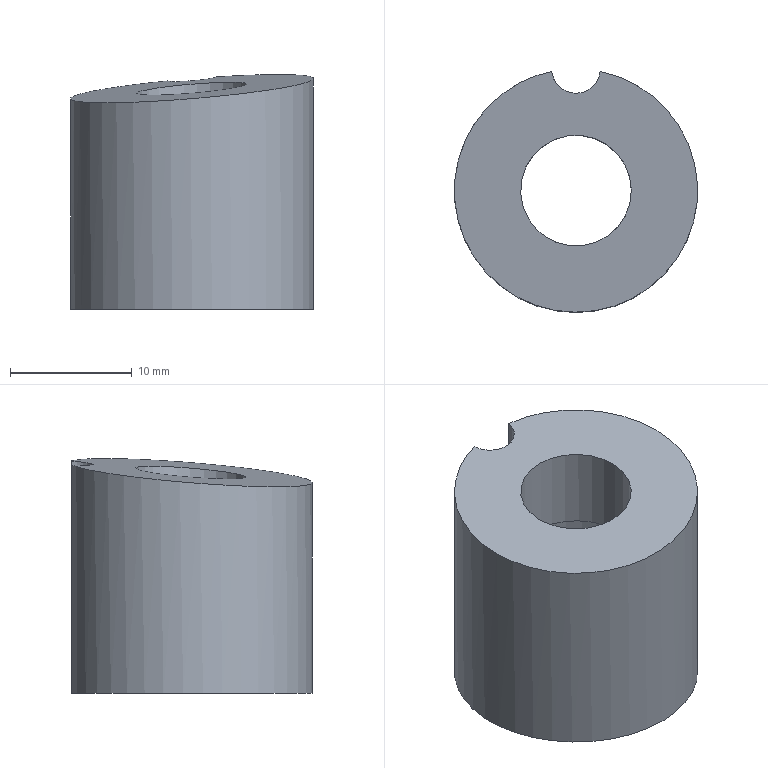Part | NX | features EKSD 20-20-10.10 2 | 1 solid | 7 faces | box 20 x 19.8 x 19.32 mm | volume 3694 mm3 | cylinder 4 | plane 3 | commonest cylinder face diameters 4 x1 9.1 x1 12.6 x1 20 x1
STEP:
#1=CARTESIAN_POINT('',(773.57,7.852,-2.));
#2=VERTEX_POINT('',#1);
#3=CARTESIAN_POINT('',(777.55,7.852,-2.));
#4=VERTEX_POINT('',#3);
#5=CARTESIAN_POINT('',(775.56,8.052,-2.));
#6=DIRECTION('',(0.,0.,1.));
#7=DIRECTION('',(1.,0.,0.));
#8=AXIS2_PLACEMENT_3D('',#5,#6,#7);
#9=CIRCLE('',#8,2.);
#10=EDGE_CURVE('',#2,#4,#9,.T.);
#11=ORIENTED_EDGE('',*,*,#10,.T.);
#12=CARTESIAN_POINT('',(775.56,-1.948,-2.));
#13=DIRECTION('',(0.,0.,1.));
#14=DIRECTION('',(1.,0.,0.));
#15=AXIS2_PLACEMENT_3D('',#12,#13,#14);
#16=CIRCLE('',#15,10.);
#17=EDGE_CURVE('',#2,#4,#16,.T.);
#18=ORIENTED_EDGE('',*,*,#17,.F.);
#19=EDGE_LOOP('',(#11,#18));
#20=FACE_BOUND('',#19,.T.);
#21=CARTESIAN_POINT('',(769.26,-1.948,-2.));
#22=VERTEX_POINT('',#21);
#23=CARTESIAN_POINT('',(775.56,-1.948,-2.));
#24=DIRECTION('',(0.,0.,-1.));
#25=DIRECTION('',(-1.,0.,0.));
#26=AXIS2_PLACEMENT_3D('',#23,#24,#25);
#27=CIRCLE('',#26,6.3);
#28=EDGE_CURVE('',#22,#22,#27,.T.);
#29=ORIENTED_EDGE('',*,*,#28,.F.);
#30=EDGE_LOOP('',(#29));
#31=FACE_BOUND('',#30,.T.);
#32=CARTESIAN_POINT('',(775.56,-1.948,-2.));
#33=DIRECTION('',(0.,0.,-1.));
#34=DIRECTION('',(-1.,0.,0.));
#35=AXIS2_PLACEMENT_3D('',#32,#33,#34);
#36=PLANE('',#35);
#37=ADVANCED_FACE('',(#20,#31),#36,.T.);
#38=CARTESIAN_POINT('',(777.55,7.852,17.123));
#39=VERTEX_POINT('',#38);
#40=CARTESIAN_POINT('',(773.57,7.852,16.794));
#41=VERTEX_POINT('',#40);
#42=CARTESIAN_POINT('',(775.56,8.052,16.975));
#43=DIRECTION('',(0.08207,0.08131,-0.9933));
#44=DIRECTION('',(-0.7057,-0.6991,-0.1155));
#45=AXIS2_PLACEMENT_3D('',#42,#43,#44);
#46=ELLIPSE('',#45,2.013,2.);
#47=EDGE_CURVE('',#39,#41,#46,.T.);
#48=ORIENTED_EDGE('',*,*,#47,.T.);
#49=CARTESIAN_POINT('',(775.56,-1.948,16.157));
#50=DIRECTION('',(0.08207,0.08131,-0.9933));
#51=DIRECTION('',(-0.7057,-0.6991,-0.1155));
#52=AXIS2_PLACEMENT_3D('',#49,#50,#51);
#53=ELLIPSE('',#52,10.067,10.);
#54=EDGE_CURVE('',#39,#41,#53,.T.);
#55=ORIENTED_EDGE('',*,*,#54,.F.);
#56=EDGE_LOOP('',(#48,#55));
#57=FACE_BOUND('',#56,.T.);
#58=CARTESIAN_POINT('',(772.328,-5.151,15.627));
#59=VERTEX_POINT('',#58);
#60=CARTESIAN_POINT('',(775.56,-1.948,16.157));
#61=DIRECTION('',(0.08207,0.08131,-0.9933));
#62=DIRECTION('',(-0.7057,-0.6991,-0.1155));
#63=AXIS2_PLACEMENT_3D('',#60,#61,#62);
#64=ELLIPSE('',#63,4.581,4.55);
#65=EDGE_CURVE('',#59,#59,#64,.F.);
#66=ORIENTED_EDGE('',*,*,#65,.F.);
#67=EDGE_LOOP('',(#66));
#68=FACE_BOUND('',#67,.T.);
#69=CARTESIAN_POINT('',(769.017,-96.065,7.912));
#70=DIRECTION('',(0.08207,0.08131,-0.9933));
#71=DIRECTION('',(0.9966,-0.01117,0.08143));
#72=AXIS2_PLACEMENT_3D('',#69,#70,#71);
#73=PLANE('',#72);
#74=ADVANCED_FACE('',(#57,#68),#73,.F.);
#75=CARTESIAN_POINT('',(777.55,7.852,8.));
#76=DIRECTION('',(0.,0.,-1.));
#77=VECTOR('',#76,1000.);
#78=LINE('',#75,#77);
#79=EDGE_CURVE('',#39,#4,#78,.T.);
#80=ORIENTED_EDGE('',*,*,#79,.F.);
#81=ORIENTED_EDGE('',*,*,#54,.T.);
#82=CARTESIAN_POINT('',(773.57,7.852,8.));
#83=DIRECTION('',(0.,0.,-1.));
#84=VECTOR('',#83,1000.);
#85=LINE('',#82,#84);
#86=EDGE_CURVE('',#2,#41,#85,.F.);
#87=ORIENTED_EDGE('',*,*,#86,.F.);
#88=ORIENTED_EDGE('',*,*,#17,.T.);
#89=EDGE_LOOP('',(#80,#81,#87,#88));
#90=FACE_BOUND('',#89,.T.);
#91=CARTESIAN_POINT('',(775.56,-1.948,18.));
#92=DIRECTION('',(0.,0.,-1.));
#93=DIRECTION('',(-1.,0.,0.));
#94=AXIS2_PLACEMENT_3D('',#91,#92,#93);
#95=CYLINDRICAL_SURFACE('',#94,10.);
#96=ADVANCED_FACE('',(#90),#95,.T.);
#97=CARTESIAN_POINT('',(780.11,-1.948,10.));
#98=VERTEX_POINT('',#97);
#99=CARTESIAN_POINT('',(775.56,-1.948,10.));
#100=DIRECTION('',(0.,0.,1.));
#101=DIRECTION('',(1.,0.,0.));
#102=AXIS2_PLACEMENT_3D('',#99,#100,#101);
#103=CIRCLE('',#102,4.55);
#104=EDGE_CURVE('',#98,#98,#103,.F.);
#105=ORIENTED_EDGE('',*,*,#104,.T.);
#106=EDGE_LOOP('',(#105));
#107=FACE_BOUND('',#106,.T.);
#108=ORIENTED_EDGE('',*,*,#65,.T.);
#109=EDGE_LOOP('',(#108));
#110=FACE_BOUND('',#109,.T.);
#111=CARTESIAN_POINT('',(775.56,-1.948,19.));
#112=DIRECTION('',(0.,0.,-1.));
#113=DIRECTION('',(-1.,0.,0.));
#114=AXIS2_PLACEMENT_3D('',#111,#112,#113);
#115=CYLINDRICAL_SURFACE('',#114,4.55);
#116=ADVANCED_FACE('',(#107,#110),#115,.F.);
#117=CARTESIAN_POINT('',(769.26,-1.948,10.));
#118=VERTEX_POINT('',#117);
#119=CARTESIAN_POINT('',(775.56,-1.948,10.));
#120=DIRECTION('',(0.,0.,-1.));
#121=DIRECTION('',(-1.,0.,0.));
#122=AXIS2_PLACEMENT_3D('',#119,#120,#121);
#123=CIRCLE('',#122,6.3);
#124=EDGE_CURVE('',#118,#118,#123,.T.);
#125=ORIENTED_EDGE('',*,*,#124,.T.);
#126=EDGE_LOOP('',(#125));
#127=FACE_BOUND('',#126,.T.);
#128=ORIENTED_EDGE('',*,*,#104,.F.);
#129=EDGE_LOOP('',(#128));
#130=FACE_BOUND('',#129,.T.);
#131=CARTESIAN_POINT('',(775.56,-1.948,10.));
#132=DIRECTION('',(0.,0.,1.));
#133=DIRECTION('',(1.,0.,0.));
#134=AXIS2_PLACEMENT_3D('',#131,#132,#133);
#135=PLANE('',#134);
#136=ADVANCED_FACE('',(#127,#130),#135,.F.);
#137=ORIENTED_EDGE('',*,*,#28,.T.);
#138=EDGE_LOOP('',(#137));
#139=FACE_BOUND('',#138,.T.);
#140=ORIENTED_EDGE('',*,*,#124,.F.);
#141=EDGE_LOOP('',(#140));
#142=FACE_BOUND('',#141,.T.);
#143=CARTESIAN_POINT('',(775.56,-1.948,10.));
#144=DIRECTION('',(0.,0.,-1.));
#145=DIRECTION('',(-1.,0.,0.));
#146=AXIS2_PLACEMENT_3D('',#143,#144,#145);
#147=CYLINDRICAL_SURFACE('',#146,6.3);
#148=ADVANCED_FACE('',(#139,#142),#147,.F.);
#149=ORIENTED_EDGE('',*,*,#79,.T.);
#150=ORIENTED_EDGE('',*,*,#10,.F.);
#151=ORIENTED_EDGE('',*,*,#86,.T.);
#152=ORIENTED_EDGE('',*,*,#47,.F.);
#153=EDGE_LOOP('',(#149,#150,#151,#152));
#154=FACE_BOUND('',#153,.T.);
#155=CARTESIAN_POINT('',(775.56,8.052,18.));
#156=DIRECTION('',(0.,0.,-1.));
#157=DIRECTION('',(-1.,0.,0.));
#158=AXIS2_PLACEMENT_3D('',#155,#156,#157);
#159=CYLINDRICAL_SURFACE('',#158,2.);
#160=ADVANCED_FACE('',(#154),#159,.F.);
#161=CLOSED_SHELL('',(#37,#74,#96,#116,#136,#148,#160));
#162=MANIFOLD_SOLID_BREP('',#161);
#163=(LENGTH_UNIT()NAMED_UNIT(*)SI_UNIT(.MILLI.,.METRE.));
#164=UNCERTAINTY_MEASURE_WITH_UNIT(LENGTH_MEASURE(0.00001),#163,'','');
#165=(NAMED_UNIT(*)PLANE_ANGLE_UNIT()SI_UNIT($,.RADIAN.));
#166=(NAMED_UNIT(*)SI_UNIT($,.STERADIAN.)SOLID_ANGLE_UNIT());
#167=(GEOMETRIC_REPRESENTATION_CONTEXT(3)GLOBAL_UNCERTAINTY_ASSIGNED_CONTEXT((#164))GLOBAL_UNIT_ASSIGNED_CONTEXT((#163,#165,#166))REPRESENTATION_CONTEXT('',''));
#168=ADVANCED_BREP_SHAPE_REPRESENTATION('',(#162),#167);